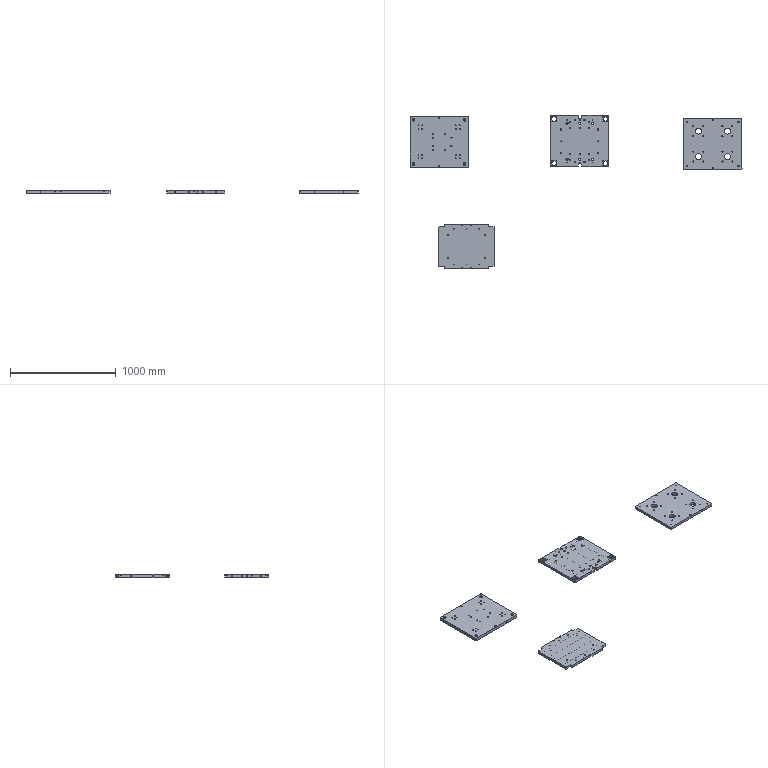NC program | Mastercam | posted with a generic post | part box 3140 x 1452 x 30 mm
Lines 17234 to 18407 of 22248, first 1084 of 1174 lines:
N4000 T12 M6
N4010 G0 G90 G17 G54 X-256.12 Y210.2 A0. S6000 M3
N4020 G43 H12 Z50. M8
N4030 Z1.
N4040 G1 Z-24.85 F600.
N4050 X-257.32 F1000.
N4060 G3 X-258.52 Y209. I0. J-1.2
N4070 X-242. Y192.48 I16.52 J0.
N4080 X-225.48 Y209. I0. J16.52
N4090 X-242. Y225.52 I-16.52 J0.
N4100 X-258.52 Y209. I0. J-16.52
N4110 X-258.512 Y208.5 I16.52 J0.
N4120 X-257.313 Y207.336 I1.199 J.036
N4130 X-257.277 Y207.337 I0. J1.2
N4140 G1 X-256.077 Y207.373
N4150 X-256.14 Y210.2
N4160 X-257.34
N4170 G3 X-258.54 Y209. I0. J-1.2
N4180 X-242. Y192.46 I16.54 J0.
N4190 X-225.46 Y209. I0. J16.54
N4200 X-242. Y225.54 I-16.54 J0.
N4210 X-258.54 Y209. I0. J-16.54
N4220 X-258.532 Y208.5 I16.54 J0.
N4230 X-257.333 Y207.336 I1.199 J.036
N4240 X-257.297 Y207.337 I0. J1.2
N4250 G1 X-256.097 Y207.373
N4260 G0 Z50.
N4270 X227.88 Y210.2
N4280 Z1.
N4290 G1 Z-24.85 F600.
N4300 X226.68 F1000.
N4310 G3 X225.48 Y209. I0. J-1.2
N4320 X242. Y192.48 I16.52 J0.
N4330 X258.52 Y209. I0. J16.52
N4340 X242. Y225.52 I-16.52 J0.
N4350 X225.48 Y209. I0. J-16.52
N4360 X225.488 Y208.5 I16.52 J0.
N4370 X226.687 Y207.336 I1.199 J.036
N4380 X226.723 Y207.337 I0. J1.2
N4390 G1 X227.923 Y207.373
N4400 X227.86 Y210.2
N4410 X226.66
N4420 G3 X225.46 Y209. I0. J-1.2
N4430 X242. Y192.46 I16.54 J0.
N4440 X258.54 Y209. I0. J16.54
N4450 X242. Y225.54 I-16.54 J0.
N4460 X225.46 Y209. I0. J-16.54
N4470 X225.468 Y208.5 I16.54 J0.
N4480 X226.667 Y207.336 I1.199 J.036
N4490 X226.703 Y207.337 I0. J1.2
N4500 G1 X227.903 Y207.373
N4510 G0 Z50.
N4520 X227.88 Y-207.8
N4530 Z1.
N4540 G1 Z-24.85 F600.
N4550 X226.68 F1000.
N4560 G3 X225.48 Y-209. I0. J-1.2
N4570 X242. Y-225.52 I16.52 J0.
N4580 X258.52 Y-209. I0. J16.52
N4590 X242. Y-192.48 I-16.52 J0.
N4600 X225.48 Y-209. I0. J-16.52
N4610 X225.488 Y-209.5 I16.52 J0.
N4620 X226.687 Y-210.664 I1.199 J.036
N4630 X226.723 Y-210.663 I0. J1.2
N4640 G1 X227.923 Y-210.627
N4650 X227.86 Y-207.8
N4660 X226.66
N4670 G3 X225.46 Y-209. I0. J-1.2
N4680 X242. Y-225.54 I16.54 J0.
N4690 X258.54 Y-209. I0. J16.54
N4700 X242. Y-192.46 I-16.54 J0.
N4710 X225.46 Y-209. I0. J-16.54
N4720 X225.468 Y-209.5 I16.54 J0.
N4730 X226.667 Y-210.664 I1.199 J.036
N4740 X226.703 Y-210.663 I0. J1.2
N4750 G1 X227.903 Y-210.627
N4760 G0 Z50.
N4770 X-256.12 Y-207.8
N4780 Z1.
N4790 G1 Z-24.85 F600.
N4800 X-257.32 F1000.
N4810 G3 X-258.52 Y-209. I0. J-1.2
N4820 X-242. Y-225.52 I16.52 J0.
N4830 X-225.48 Y-209. I0. J16.52
N4840 X-242. Y-192.48 I-16.52 J0.
N4850 X-258.52 Y-209. I0. J-16.52
N4860 X-258.512 Y-209.5 I16.52 J0.
N4870 X-257.313 Y-210.664 I1.199 J.036
N4880 X-257.277 Y-210.663 I0. J1.2
N4890 G1 X-256.077 Y-210.627
N4900 X-256.14 Y-207.8
N4910 X-257.34
N4920 G3 X-258.54 Y-209. I0. J-1.2
N4930 X-242. Y-225.54 I16.54 J0.
N4940 X-225.46 Y-209. I0. J16.54
N4950 X-242. Y-192.46 I-16.54 J0.
N4960 X-258.54 Y-209. I0. J-16.54
N4970 X-258.532 Y-209.5 I16.54 J0.
N4980 X-257.333 Y-210.664 I1.199 J.036
N4990 X-257.297 Y-210.663 I0. J1.2
N5000 G1 X-256.097 Y-210.627
N5010 G0 Z50.
N5020 X-124.18 Y170.
N5030 Z1.2
N5040 G1 Z.2 F600.
N5050 G3 X-120. Y165.82 Z.025 I4.18 J0. F2000.
N5060 X-115.82 Y170. Z-.15 I0. J4.18
N5070 X-120. Y174.18 Z-.325 I-4.18 J0.
N5080 X-124.18 Y170. Z-.5 I0. J-4.18
N5090 X-120. Y165.82 Z-.675 I4.18 J0.
N5100 X-115.82 Y170. Z-.85 I0. J4.18
N5110 X-120. Y174.18 Z-1.025 I-4.18 J0.
N5120 X-124.18 Y170. Z-1.2 I0. J-4.18
N5130 X-120. Y165.82 Z-1.375 I4.18 J0.
N5140 X-115.82 Y170. Z-1.55 I0. J4.18
N5150 X-120. Y174.18 Z-1.725 I-4.18 J0.
N5160 X-124.18 Y170. Z-1.9 I0. J-4.18
N5170 X-120. Y165.82 Z-2.075 I4.18 J0.
N5180 X-115.82 Y170. Z-2.25 I0. J4.18
N5190 X-120. Y174.18 Z-2.425 I-4.18 J0.
N5200 X-124.18 Y170. Z-2.6 I0. J-4.18
N5210 X-120. Y165.82 Z-2.775 I4.18 J0.
N5220 X-115.82 Y170. Z-2.95 I0. J4.18
N5230 X-120. Y174.18 Z-3.125 I-4.18 J0.
N5240 X-124.18 Y170. Z-3.3 I0. J-4.18
N5250 X-120. Y165.82 Z-3.475 I4.18 J0.
N5260 X-115.82 Y170. Z-3.65 I0. J4.18
N5270 X-120. Y174.18 Z-3.825 I-4.18 J0.
N5280 X-124.18 Y170. Z-4. I0. J-4.18
N5290 X-120. Y165.82 Z-4.175 I4.18 J0.
N5300 X-115.82 Y170. Z-4.35 I0. J4.18
N5310 X-120. Y174.18 Z-4.525 I-4.18 J0.
N5320 X-124.18 Y170. Z-4.7 I0. J-4.18
N5330 X-120. Y165.82 Z-4.875 I4.18 J0.
N5340 X-115.82 Y170. Z-5.05 I0. J4.18
N5350 X-120. Y174.18 Z-5.225 I-4.18 J0.
N5360 X-124.18 Y170. Z-5.4 I0. J-4.18
N5370 X-120. Y165.82 Z-5.575 I4.18 J0.
N5380 X-115.82 Y170. Z-5.75 I0. J4.18
N5390 X-120. Y174.18 Z-5.925 I-4.18 J0.
N5400 X-124.18 Y170. Z-6.1 I0. J-4.18
N5410 X-120. Y165.82 Z-6.275 I4.18 J0.
N5420 X-115.82 Y170. Z-6.45 I0. J4.18
N5430 X-120. Y174.18 Z-6.625 I-4.18 J0.
N5440 X-124.18 Y170. Z-6.8 I0. J-4.18
N5450 X-120. Y165.82 Z-6.975 I4.18 J0.
N5460 X-115.82 Y170. Z-7.15 I0. J4.18
N5470 X-120. Y174.18 Z-7.325 I-4.18 J0.
N5480 X-124.18 Y170. Z-7.5 I0. J-4.18
N5490 X-120. Y165.82 Z-7.675 I4.18 J0.
N5500 X-115.82 Y170. Z-7.85 I0. J4.18
N5510 X-120. Y174.18 Z-8.025 I-4.18 J0.
N5520 X-124.18 Y170. Z-8.2 I0. J-4.18
N5530 X-120. Y165.82 Z-8.375 I4.18 J0.
N5540 X-115.82 Y170. Z-8.55 I0. J4.18
N5550 X-120. Y174.18 Z-8.725 I-4.18 J0.
N5560 X-124.18 Y170. Z-8.9 I0. J-4.18
N5570 X-120. Y165.82 Z-9.075 I4.18 J0.
N5580 X-115.82 Y170. Z-9.25 I0. J4.18
N5590 X-120. Y174.18 Z-9.425 I-4.18 J0.
N5600 X-124.18 Y170. Z-9.6 I0. J-4.18
N5610 X-120. Y165.82 Z-9.775 I4.18 J0.
N5620 X-115.82 Y170. Z-9.95 I0. J4.18
N5630 X-120. Y174.18 Z-10.125 I-4.18 J0.
N5640 X-124.18 Y170. Z-10.3 I0. J-4.18
N5650 X-120. Y165.82 Z-10.475 I4.18 J0.
N5660 X-115.82 Y170. Z-10.65 I0. J4.18
N5670 X-120. Y174.18 Z-10.825 I-4.18 J0.
N5680 X-124.18 Y170. Z-11. I0. J-4.18
N5690 X-120. Y165.82 Z-11.175 I4.18 J0.
N5700 X-115.82 Y170. Z-11.35 I0. J4.18
N5710 X-120. Y174.18 Z-11.525 I-4.18 J0.
N5720 X-124.18 Y170. Z-11.7 I0. J-4.18
N5730 X-120. Y165.82 Z-11.875 I4.18 J0.
N5740 X-115.82 Y170. Z-12.05 I0. J4.18
N5750 X-120. Y174.18 Z-12.225 I-4.18 J0.
N5760 X-124.18 Y170. Z-12.4 I0. J-4.18
N5770 X-120. Y165.82 Z-12.575 I4.18 J0.
N5780 X-115.82 Y170. Z-12.75 I0. J4.18
N5790 X-120. Y174.18 Z-12.925 I-4.18 J0.
N5800 X-124.18 Y170. Z-13.1 I0. J-4.18
N5810 X-120. Y165.82 Z-13.275 I4.18 J0.
N5820 X-115.82 Y170. Z-13.45 I0. J4.18
N5830 X-120. Y174.18 Z-13.625 I-4.18 J0.
N5840 X-124.18 Y170. Z-13.8 I0. J-4.18
N5850 X-120. Y165.82 Z-13.975 I4.18 J0.
N5860 X-115.82 Y170. Z-14.15 I0. J4.18
N5870 X-120. Y174.18 Z-14.325 I-4.18 J0.
N5880 X-124.18 Y170. Z-14.5 I0. J-4.18
N5890 X-120. Y165.82 Z-14.675 I4.18 J0.
N5900 X-115.82 Y170. Z-14.85 I0. J4.18
N5910 X-120. Y174.18 Z-15.025 I-4.18 J0.
N5920 X-124.18 Y170. Z-15.2 I0. J-4.18
N5930 X-120. Y165.82 Z-15.375 I4.18 J0.
N5940 X-115.82 Y170. Z-15.55 I0. J4.18
N5950 X-120. Y174.18 Z-15.725 I-4.18 J0.
N5960 X-124.18 Y170. Z-15.9 I0. J-4.18
N5970 X-120. Y165.82 Z-16.075 I4.18 J0.
N5980 X-115.82 Y170. Z-16.25 I0. J4.18
N5990 X-120. Y174.18 Z-16.425 I-4.18 J0.
N6000 X-124.18 Y170. Z-16.6 I0. J-4.18
N6010 X-120. Y165.82 Z-16.775 I4.18 J0.
N6020 X-115.82 Y170. Z-16.95 I0. J4.18
N6030 X-120. Y174.18 Z-17.125 I-4.18 J0.
N6040 X-124.18 Y170. Z-17.3 I0. J-4.18
N6050 X-120. Y165.82 Z-17.475 I4.18 J0.
N6060 X-115.82 Y170. Z-17.65 I0. J4.18
N6070 X-120. Y174.18 Z-17.825 I-4.18 J0.
N6080 X-124.18 Y170. Z-18. I0. J-4.18
N6090 X-120. Y165.82 Z-18.175 I4.18 J0.
N6100 X-115.82 Y170. Z-18.35 I0. J4.18
N6110 X-120. Y174.18 Z-18.525 I-4.18 J0.
N6120 X-124.18 Y170. Z-18.7 I0. J-4.18
N6130 X-120. Y165.82 Z-18.875 I4.18 J0.
N6140 X-115.82 Y170. Z-19.05 I0. J4.18
N6150 X-120. Y174.18 Z-19.225 I-4.18 J0.
N6160 X-124.18 Y170. Z-19.4 I0. J-4.18
N6170 X-120. Y165.82 Z-19.575 I4.18 J0.
N6180 X-115.82 Y170. Z-19.75 I0. J4.18
N6190 X-120. Y174.18 Z-19.925 I-4.18 J0.
N6200 X-124.18 Y170. Z-20.1 I0. J-4.18
N6210 X-120. Y165.82 Z-20.275 I4.18 J0.
N6220 X-115.82 Y170. Z-20.45 I0. J4.18
N6230 X-120. Y174.18 Z-20.625 I-4.18 J0.
N6240 X-124.18 Y170. Z-20.8 I0. J-4.18
N6250 X-120. Y165.82 Z-20.975 I4.18 J0.
N6260 X-115.82 Y170. Z-21.15 I0. J4.18
N6270 X-120. Y174.18 Z-21.325 I-4.18 J0.
N6280 X-124.18 Y170. Z-21.5 I0. J-4.18
N6290 X-120. Y165.82 Z-21.675 I4.18 J0.
N6300 X-115.82 Y170. Z-21.85 I0. J4.18
N6310 X-120. Y174.18 Z-22.025 I-4.18 J0.
N6320 X-124.18 Y170. Z-22.2 I0. J-4.18
N6330 X-120. Y165.82 Z-22.375 I4.18 J0.
N6340 X-115.82 Y170. Z-22.55 I0. J4.18
N6350 X-120. Y174.18 Z-22.725 I-4.18 J0.
N6360 X-124.18 Y170. Z-22.9 I0. J-4.18
N6370 X-120. Y165.82 Z-23.075 I4.18 J0.
N6380 X-115.82 Y170. Z-23.25 I0. J4.18
N6390 X-120. Y174.18 Z-23.425 I-4.18 J0.
N6400 X-124.18 Y170. Z-23.6 I0. J-4.18
N6410 X-120. Y165.82 Z-23.775 I4.18 J0.
N6420 X-115.82 Y170. Z-23.95 I0. J4.18
N6430 X-120. Y174.18 Z-24.125 I-4.18 J0.
N6440 X-124.18 Y170. Z-24.3 I0. J-4.18
N6450 X-120. Y165.82 Z-24.475 I4.18 J0.
N6460 X-115.82 Y170. Z-24.65 I0. J4.18
N6470 X-120. Y174.18 Z-24.825 I-4.18 J0.
N6480 X-120.93 Y174.075 Z-24.85 I0. J-4.18
N6490 X-124.18 Y170. I.93 J-4.075
N6500 X-120. Y165.82 I4.18 J0.
N6510 X-115.82 Y170. I0. J4.18
N6520 X-120. Y174.18 I-4.18 J0.
N6530 X-121.41 Y173.935 I0. J-4.18
N6540 G0 Z50.
N6550 X-4.18 Y170.
N6560 Z1.2
N6570 G1 Z.2 F600.
N6580 G3 X0. Y165.82 Z.025 I4.18 J0. F2000.
N6590 X4.18 Y170. Z-.15 I0. J4.18
N6600 X0. Y174.18 Z-.325 I-4.18 J0.
N6610 X-4.18 Y170. Z-.5 I0. J-4.18
N6620 X0. Y165.82 Z-.675 I4.18 J0.
N6630 X4.18 Y170. Z-.85 I0. J4.18
N6640 X0. Y174.18 Z-1.025 I-4.18 J0.
N6650 X-4.18 Y170. Z-1.2 I0. J-4.18
N6660 X0. Y165.82 Z-1.375 I4.18 J0.
N6670 X4.18 Y170. Z-1.55 I0. J4.18
N6680 X0. Y174.18 Z-1.725 I-4.18 J0.
N6690 X-4.18 Y170. Z-1.9 I0. J-4.18
N6700 X0. Y165.82 Z-2.075 I4.18 J0.
N6710 X4.18 Y170. Z-2.25 I0. J4.18
N6720 X0. Y174.18 Z-2.425 I-4.18 J0.
N6730 X-4.18 Y170. Z-2.6 I0. J-4.18
N6740 X0. Y165.82 Z-2.775 I4.18 J0.
N6750 X4.18 Y170. Z-2.95 I0. J4.18
N6760 X0. Y174.18 Z-3.125 I-4.18 J0.
N6770 X-4.18 Y170. Z-3.3 I0. J-4.18
N6780 X0. Y165.82 Z-3.475 I4.18 J0.
N6790 X4.18 Y170. Z-3.65 I0. J4.18
N6800 X0. Y174.18 Z-3.825 I-4.18 J0.
N6810 X-4.18 Y170. Z-4. I0. J-4.18
N6820 X0. Y165.82 Z-4.175 I4.18 J0.
N6830 X4.18 Y170. Z-4.35 I0. J4.18
N6840 X0. Y174.18 Z-4.525 I-4.18 J0.
N6850 X-4.18 Y170. Z-4.7 I0. J-4.18
N6860 X0. Y165.82 Z-4.875 I4.18 J0.
N6870 X4.18 Y170. Z-5.05 I0. J4.18
N6880 X0. Y174.18 Z-5.225 I-4.18 J0.
N6890 X-4.18 Y170. Z-5.4 I0. J-4.18
N6900 X0. Y165.82 Z-5.575 I4.18 J0.
N6910 X4.18 Y170. Z-5.75 I0. J4.18
N6920 X0. Y174.18 Z-5.925 I-4.18 J0.
N6930 X-4.18 Y170. Z-6.1 I0. J-4.18
N6940 X0. Y165.82 Z-6.275 I4.18 J0.
N6950 X4.18 Y170. Z-6.45 I0. J4.18
N6960 X0. Y174.18 Z-6.625 I-4.18 J0.
N6970 X-4.18 Y170. Z-6.8 I0. J-4.18
N6980 X0. Y165.82 Z-6.975 I4.18 J0.
N6990 X4.18 Y170. Z-7.15 I0. J4.18
N7000 X0. Y174.18 Z-7.325 I-4.18 J0.
N7010 X-4.18 Y170. Z-7.5 I0. J-4.18
N7020 X0. Y165.82 Z-7.675 I4.18 J0.
N7030 X4.18 Y170. Z-7.85 I0. J4.18
N7040 X0. Y174.18 Z-8.025 I-4.18 J0.
N7050 X-4.18 Y170. Z-8.2 I0. J-4.18
N7060 X0. Y165.82 Z-8.375 I4.18 J0.
N7070 X4.18 Y170. Z-8.55 I0. J4.18
N7080 X0. Y174.18 Z-8.725 I-4.18 J0.
N7090 X-4.18 Y170. Z-8.9 I0. J-4.18
N7100 X0. Y165.82 Z-9.075 I4.18 J0.
N7110 X4.18 Y170. Z-9.25 I0. J4.18
N7120 X0. Y174.18 Z-9.425 I-4.18 J0.
N7130 X-4.18 Y170. Z-9.6 I0. J-4.18
N7140 X0. Y165.82 Z-9.775 I4.18 J0.
N7150 X4.18 Y170. Z-9.95 I0. J4.18
N7160 X0. Y174.18 Z-10.125 I-4.18 J0.
N7170 X-4.18 Y170. Z-10.3 I0. J-4.18
N7180 X0. Y165.82 Z-10.475 I4.18 J0.
N7190 X4.18 Y170. Z-10.65 I0. J4.18
N7200 X0. Y174.18 Z-10.825 I-4.18 J0.
N7210 X-4.18 Y170. Z-11. I0. J-4.18
N7220 X0. Y165.82 Z-11.175 I4.18 J0.
N7230 X4.18 Y170. Z-11.35 I0. J4.18
N7240 X0. Y174.18 Z-11.525 I-4.18 J0.
N7250 X-4.18 Y170. Z-11.7 I0. J-4.18
N7260 X0. Y165.82 Z-11.875 I4.18 J0.
N7270 X4.18 Y170. Z-12.05 I0. J4.18
N7280 X0. Y174.18 Z-12.225 I-4.18 J0.
N7290 X-4.18 Y170. Z-12.4 I0. J-4.18
N7300 X0. Y165.82 Z-12.575 I4.18 J0.
N7310 X4.18 Y170. Z-12.75 I0. J4.18
N7320 X0. Y174.18 Z-12.925 I-4.18 J0.
N7330 X-4.18 Y170. Z-13.1 I0. J-4.18
N7340 X0. Y165.82 Z-13.275 I4.18 J0.
N7350 X4.18 Y170. Z-13.45 I0. J4.18
N7360 X0. Y174.18 Z-13.625 I-4.18 J0.
N7370 X-4.18 Y170. Z-13.8 I0. J-4.18
N7380 X0. Y165.82 Z-13.975 I4.18 J0.
N7390 X4.18 Y170. Z-14.15 I0. J4.18
N7400 X0. Y174.18 Z-14.325 I-4.18 J0.
N7410 X-4.18 Y170. Z-14.5 I0. J-4.18
N7420 X0. Y165.82 Z-14.675 I4.18 J0.
N7430 X4.18 Y170. Z-14.85 I0. J4.18
N7440 X0. Y174.18 Z-15.025 I-4.18 J0.
N7450 X-4.18 Y170. Z-15.2 I0. J-4.18
N7460 X0. Y165.82 Z-15.375 I4.18 J0.
N7470 X4.18 Y170. Z-15.55 I0. J4.18
N7480 X0. Y174.18 Z-15.725 I-4.18 J0.
N7490 X-4.18 Y170. Z-15.9 I0. J-4.18
N7500 X0. Y165.82 Z-16.075 I4.18 J0.
N7510 X4.18 Y170. Z-16.25 I0. J4.18
N7520 X0. Y174.18 Z-16.425 I-4.18 J0.
N7530 X-4.18 Y170. Z-16.6 I0. J-4.18
N7540 X0. Y165.82 Z-16.775 I4.18 J0.
N7550 X4.18 Y170. Z-16.95 I0. J4.18
N7560 X0. Y174.18 Z-17.125 I-4.18 J0.
N7570 X-4.18 Y170. Z-17.3 I0. J-4.18
N7580 X0. Y165.82 Z-17.475 I4.18 J0.
N7590 X4.18 Y170. Z-17.65 I0. J4.18
N7600 X0. Y174.18 Z-17.825 I-4.18 J0.
N7610 X-4.18 Y170. Z-18. I0. J-4.18
N7620 X0. Y165.82 Z-18.175 I4.18 J0.
N7630 X4.18 Y170. Z-18.35 I0. J4.18
N7640 X0. Y174.18 Z-18.525 I-4.18 J0.
N7650 X-4.18 Y170. Z-18.7 I0. J-4.18
N7660 X0. Y165.82 Z-18.875 I4.18 J0.
N7670 X4.18 Y170. Z-19.05 I0. J4.18
N7680 X0. Y174.18 Z-19.225 I-4.18 J0.
N7690 X-4.18 Y170. Z-19.4 I0. J-4.18
N7700 X0. Y165.82 Z-19.575 I4.18 J0.
N7710 X4.18 Y170. Z-19.75 I0. J4.18
N7720 X0. Y174.18 Z-19.925 I-4.18 J0.
N7730 X-4.18 Y170. Z-20.1 I0. J-4.18
N7740 X0. Y165.82 Z-20.275 I4.18 J0.
N7750 X4.18 Y170. Z-20.45 I0. J4.18
N7760 X0. Y174.18 Z-20.625 I-4.18 J0.
N7770 X-4.18 Y170. Z-20.8 I0. J-4.18
N7780 X0. Y165.82 Z-20.975 I4.18 J0.
N7790 X4.18 Y170. Z-21.15 I0. J4.18
N7800 X0. Y174.18 Z-21.325 I-4.18 J0.
N7810 X-4.18 Y170. Z-21.5 I0. J-4.18
N7820 X0. Y165.82 Z-21.675 I4.18 J0.
N7830 X4.18 Y170. Z-21.85 I0. J4.18
N7840 X0. Y174.18 Z-22.025 I-4.18 J0.
N7850 X-4.18 Y170. Z-22.2 I0. J-4.18
N7860 X0. Y165.82 Z-22.375 I4.18 J0.
N7870 X4.18 Y170. Z-22.55 I0. J4.18
N7880 X0. Y174.18 Z-22.725 I-4.18 J0.
N7890 X-4.18 Y170. Z-22.9 I0. J-4.18
N7900 X0. Y165.82 Z-23.075 I4.18 J0.
N7910 X4.18 Y170. Z-23.25 I0. J4.18
N7920 X0. Y174.18 Z-23.425 I-4.18 J0.
N7930 X-4.18 Y170. Z-23.6 I0. J-4.18
N7940 X0. Y165.82 Z-23.775 I4.18 J0.
N7950 X4.18 Y170. Z-23.95 I0. J4.18
N7960 X0. Y174.18 Z-24.125 I-4.18 J0.
N7970 X-4.18 Y170. Z-24.3 I0. J-4.18
N7980 X0. Y165.82 Z-24.475 I4.18 J0.
N7990 X4.18 Y170. Z-24.65 I0. J4.18
N8000 X0. Y174.18 Z-24.825 I-4.18 J0.
N8010 X-.93 Y174.075 Z-24.85 I0. J-4.18
N8020 X-4.18 Y170. I.93 J-4.075
N8030 X0. Y165.82 I4.18 J0.
N8040 X4.18 Y170. I0. J4.18
N8050 X0. Y174.18 I-4.18 J0.
N8060 X-1.41 Y173.935 I0. J-4.18
N8070 G0 Z50.
N8080 X115.82 Y170.
N8090 Z1.2
N8100 G1 Z.2 F600.
N8110 G3 X120. Y165.82 Z.025 I4.18 J0. F2000.
N8120 X124.18 Y170. Z-.15 I0. J4.18
N8130 X120. Y174.18 Z-.325 I-4.18 J0.
N8140 X115.82 Y170. Z-.5 I0. J-4.18
N8150 X120. Y165.82 Z-.675 I4.18 J0.
N8160 X124.18 Y170. Z-.85 I0. J4.18
N8170 X120. Y174.18 Z-1.025 I-4.18 J0.
N8180 X115.82 Y170. Z-1.2 I0. J-4.18
N8190 X120. Y165.82 Z-1.375 I4.18 J0.
N8200 X124.18 Y170. Z-1.55 I0. J4.18
N8210 X120. Y174.18 Z-1.725 I-4.18 J0.
N8220 X115.82 Y170. Z-1.9 I0. J-4.18
N8230 X120. Y165.82 Z-2.075 I4.18 J0.
N8240 X124.18 Y170. Z-2.25 I0. J4.18
N8250 X120. Y174.18 Z-2.425 I-4.18 J0.
N8260 X115.82 Y170. Z-2.6 I0. J-4.18
N8270 X120. Y165.82 Z-2.775 I4.18 J0.
N8280 X124.18 Y170. Z-2.95 I0. J4.18
N8290 X120. Y174.18 Z-3.125 I-4.18 J0.
N8300 X115.82 Y170. Z-3.3 I0. J-4.18
N8310 X120. Y165.82 Z-3.475 I4.18 J0.
N8320 X124.18 Y170. Z-3.65 I0. J4.18
N8330 X120. Y174.18 Z-3.825 I-4.18 J0.
N8340 X115.82 Y170. Z-4. I0. J-4.18
N8350 X120. Y165.82 Z-4.175 I4.18 J0.
N8360 X124.18 Y170. Z-4.35 I0. J4.18
N8370 X120. Y174.18 Z-4.525 I-4.18 J0.
N8380 X115.82 Y170. Z-4.7 I0. J-4.18
N8390 X120. Y165.82 Z-4.875 I4.18 J0.
N8400 X124.18 Y170. Z-5.05 I0. J4.18
N8410 X120. Y174.18 Z-5.225 I-4.18 J0.
N8420 X115.82 Y170. Z-5.4 I0. J-4.18
N8430 X120. Y165.82 Z-5.575 I4.18 J0.
N8440 X124.18 Y170. Z-5.75 I0. J4.18
N8450 X120. Y174.18 Z-5.925 I-4.18 J0.
N8460 X115.82 Y170. Z-6.1 I0. J-4.18
N8470 X120. Y165.82 Z-6.275 I4.18 J0.
N8480 X124.18 Y170. Z-6.45 I0. J4.18
N8490 X120. Y174.18 Z-6.625 I-4.18 J0.
N8500 X115.82 Y170. Z-6.8 I0. J-4.18
N8510 X120. Y165.82 Z-6.975 I4.18 J0.
N8520 X124.18 Y170. Z-7.15 I0. J4.18
N8530 X120. Y174.18 Z-7.325 I-4.18 J0.
N8540 X115.82 Y170. Z-7.5 I0. J-4.18
N8550 X120. Y165.82 Z-7.675 I4.18 J0.
N8560 X124.18 Y170. Z-7.85 I0. J4.18
N8570 X120. Y174.18 Z-8.025 I-4.18 J0.
N8580 X115.82 Y170. Z-8.2 I0. J-4.18
N8590 X120. Y165.82 Z-8.375 I4.18 J0.
N8600 X124.18 Y170. Z-8.55 I0. J4.18
N8610 X120. Y174.18 Z-8.725 I-4.18 J0.
N8620 X115.82 Y170. Z-8.9 I0. J-4.18
N8630 X120. Y165.82 Z-9.075 I4.18 J0.
N8640 X124.18 Y170. Z-9.25 I0. J4.18
N8650 X120. Y174.18 Z-9.425 I-4.18 J0.
N8660 X115.82 Y170. Z-9.6 I0. J-4.18
N8670 X120. Y165.82 Z-9.775 I4.18 J0.
N8680 X124.18 Y170. Z-9.95 I0. J4.18
N8690 X120. Y174.18 Z-10.125 I-4.18 J0.
N8700 X115.82 Y170. Z-10.3 I0. J-4.18
N8710 X120. Y165.82 Z-10.475 I4.18 J0.
N8720 X124.18 Y170. Z-10.65 I0. J4.18
N8730 X120. Y174.18 Z-10.825 I-4.18 J0.
N8740 X115.82 Y170. Z-11. I0. J-4.18
N8750 X120. Y165.82 Z-11.175 I4.18 J0.
N8760 X124.18 Y170. Z-11.35 I0. J4.18
N8770 X120. Y174.18 Z-11.525 I-4.18 J0.
N8780 X115.82 Y170. Z-11.7 I0. J-4.18
N8790 X120. Y165.82 Z-11.875 I4.18 J0.
N8800 X124.18 Y170. Z-12.05 I0. J4.18
N8810 X120. Y174.18 Z-12.225 I-4.18 J0.
N8820 X115.82 Y170. Z-12.4 I0. J-4.18
N8830 X120. Y165.82 Z-12.575 I4.18 J0.
N8840 X124.18 Y170. Z-12.75 I0. J4.18
N8850 X120. Y174.18 Z-12.925 I-4.18 J0.
N8860 X115.82 Y170. Z-13.1 I0. J-4.18
N8870 X120. Y165.82 Z-13.275 I4.18 J0.
N8880 X124.18 Y170. Z-13.45 I0. J4.18
N8890 X120. Y174.18 Z-13.625 I-4.18 J0.
N8900 X115.82 Y170. Z-13.8 I0. J-4.18
N8910 X120. Y165.82 Z-13.975 I4.18 J0.
N8920 X124.18 Y170. Z-14.15 I0. J4.18
N8930 X120. Y174.18 Z-14.325 I-4.18 J0.
N8940 X115.82 Y170. Z-14.5 I0. J-4.18
N8950 X120. Y165.82 Z-14.675 I4.18 J0.
N8960 X124.18 Y170. Z-14.85 I0. J4.18
N8970 X120. Y174.18 Z-15.025 I-4.18 J0.
N8980 X115.82 Y170. Z-15.2 I0. J-4.18
N8990 X120. Y165.82 Z-15.375 I4.18 J0.
N9000 X124.18 Y170. Z-15.55 I0. J4.18
N9010 X120. Y174.18 Z-15.725 I-4.18 J0.
N9020 X115.82 Y170. Z-15.9 I0. J-4.18
N9030 X120. Y165.82 Z-16.075 I4.18 J0.
N9040 X124.18 Y170. Z-16.25 I0. J4.18
N9050 X120. Y174.18 Z-16.425 I-4.18 J0.
N9060 X115.82 Y170. Z-16.6 I0. J-4.18
N9070 X120. Y165.82 Z-16.775 I4.18 J0.
N9080 X124.18 Y170. Z-16.95 I0. J4.18
N9090 X120. Y174.18 Z-17.125 I-4.18 J0.
N9100 X115.82 Y170. Z-17.3 I0. J-4.18
N9110 X120. Y165.82 Z-17.475 I4.18 J0.
N9120 X124.18 Y170. Z-17.65 I0. J4.18
N9130 X120. Y174.18 Z-17.825 I-4.18 J0.
N9140 X115.82 Y170. Z-18. I0. J-4.18
N9150 X120. Y165.82 Z-18.175 I4.18 J0.
N9160 X124.18 Y170. Z-18.35 I0. J4.18
N9170 X120. Y174.18 Z-18.525 I-4.18 J0.
N9180 X115.82 Y170. Z-18.7 I0. J-4.18
N9190 X120. Y165.82 Z-18.875 I4.18 J0.
N9200 X124.18 Y170. Z-19.05 I0. J4.18
N9210 X120. Y174.18 Z-19.225 I-4.18 J0.
N9220 X115.82 Y170. Z-19.4 I0. J-4.18
N9230 X120. Y165.82 Z-19.575 I4.18 J0.
N9240 X124.18 Y170. Z-19.75 I0. J4.18
N9250 X120. Y174.18 Z-19.925 I-4.18 J0.
N9260 X115.82 Y170. Z-20.1 I0. J-4.18
N9270 X120. Y165.82 Z-20.275 I4.18 J0.
N9280 X124.18 Y170. Z-20.45 I0. J4.18
N9290 X120. Y174.18 Z-20.625 I-4.18 J0.
N9300 X115.82 Y170. Z-20.8 I0. J-4.18
N9310 X120. Y165.82 Z-20.975 I4.18 J0.
N9320 X124.18 Y170. Z-21.15 I0. J4.18
N9330 X120. Y174.18 Z-21.325 I-4.18 J0.
N9340 X115.82 Y170. Z-21.5 I0. J-4.18
N9350 X120. Y165.82 Z-21.675 I4.18 J0.
N9360 X124.18 Y170. Z-21.85 I0. J4.18
N9370 X120. Y174.18 Z-22.025 I-4.18 J0.
N9380 X115.82 Y170. Z-22.2 I0. J-4.18
N9390 X120. Y165.82 Z-22.375 I4.18 J0.
N9400 X124.18 Y170. Z-22.55 I0. J4.18
N9410 X120. Y174.18 Z-22.725 I-4.18 J0.
N9420 X115.82 Y170. Z-22.9 I0. J-4.18
N9430 X120. Y165.82 Z-23.075 I4.18 J0.
N9440 X124.18 Y170. Z-23.25 I0. J4.18
N9450 X120. Y174.18 Z-23.425 I-4.18 J0.
N9460 X115.82 Y170. Z-23.6 I0. J-4.18
N9470 X120. Y165.82 Z-23.775 I4.18 J0.
N9480 X124.18 Y170. Z-23.95 I0. J4.18
N9490 X120. Y174.18 Z-24.125 I-4.18 J0.
N9500 X115.82 Y170. Z-24.3 I0. J-4.18
N9510 X120. Y165.82 Z-24.475 I4.18 J0.
N9520 X124.18 Y170. Z-24.65 I0. J4.18
N9530 X120. Y174.18 Z-24.825 I-4.18 J0.
N9540 X119.07 Y174.075 Z-24.85 I0. J-4.18
N9550 X115.82 Y170. I.93 J-4.075
N9560 X120. Y165.82 I4.18 J0.
N9570 X124.18 Y170. I0. J4.18
N9580 X120. Y174.18 I-4.18 J0.
N9590 X118.59 Y173.935 I0. J-4.18
N9600 G0 Z50.
N9610 X115.82 Y-170.
N9620 Z1.2
N9630 G1 Z.2 F600.
N9640 G3 X120. Y-174.18 Z.025 I4.18 J0. F2000.
N9650 X124.18 Y-170. Z-.15 I0. J4.18
N9660 X120. Y-165.82 Z-.325 I-4.18 J0.
N9670 X115.82 Y-170. Z-.5 I0. J-4.18
N9680 X120. Y-174.18 Z-.675 I4.18 J0.
N9690 X124.18 Y-170. Z-.85 I0. J4.18
N9700 X120. Y-165.82 Z-1.025 I-4.18 J0.
N9710 X115.82 Y-170. Z-1.2 I0. J-4.18
N9720 X120. Y-174.18 Z-1.375 I4.18 J0.
N9730 X124.18 Y-170. Z-1.55 I0. J4.18
N9740 X120. Y-165.82 Z-1.725 I-4.18 J0.
N9750 X115.82 Y-170. Z-1.9 I0. J-4.18
N9760 X120. Y-174.18 Z-2.075 I4.18 J0.
N9770 X124.18 Y-170. Z-2.25 I0. J4.18
N9780 X120. Y-165.82 Z-2.425 I-4.18 J0.
N9790 X115.82 Y-170. Z-2.6 I0. J-4.18
N9800 X120. Y-174.18 Z-2.775 I4.18 J0.
N9810 X124.18 Y-170. Z-2.95 I0. J4.18
N9820 X120. Y-165.82 Z-3.125 I-4.18 J0.
N9830 X115.82 Y-170. Z-3.3 I0. J-4.18
N9840 X120. Y-174.18 Z-3.475 I4.18 J0.
N9850 X124.18 Y-170. Z-3.65 I0. J4.18
N9860 X120. Y-165.82 Z-3.825 I-4.18 J0.
N9870 X115.82 Y-170. Z-4. I0. J-4.18
N9880 X120. Y-174.18 Z-4.175 I4.18 J0.
N9890 X124.18 Y-170. Z-4.35 I0. J4.18
N9900 X120. Y-165.82 Z-4.525 I-4.18 J0.
N9910 X115.82 Y-170. Z-4.7 I0. J-4.18
N9920 X120. Y-174.18 Z-4.875 I4.18 J0.
N9930 X124.18 Y-170. Z-5.05 I0. J4.18
N9940 X120. Y-165.82 Z-5.225 I-4.18 J0.
N9950 X115.82 Y-170. Z-5.4 I0. J-4.18
N9960 X120. Y-174.18 Z-5.575 I4.18 J0.
N9970 X124.18 Y-170. Z-5.75 I0. J4.18
N9980 X120. Y-165.82 Z-5.925 I-4.18 J0.
N9990 X115.82 Y-170. Z-6.1 I0. J-4.18
N100 X120. Y-174.18 Z-6.275 I4.18 J0.
N110 X124.18 Y-170. Z-6.45 I0. J4.18
N120 X120. Y-165.82 Z-6.625 I-4.18 J0.
N130 X115.82 Y-170. Z-6.8 I0. J-4.18
N140 X120. Y-174.18 Z-6.975 I4.18 J0.
N150 X124.18 Y-170. Z-7.15 I0. J4.18
N160 X120. Y-165.82 Z-7.325 I-4.18 J0.
N170 X115.82 Y-170. Z-7.5 I0. J-4.18
N180 X120. Y-174.18 Z-7.675 I4.18 J0.
N190 X124.18 Y-170. Z-7.85 I0. J4.18
N200 X120. Y-165.82 Z-8.025 I-4.18 J0.
N210 X115.82 Y-170. Z-8.2 I0. J-4.18
N220 X120. Y-174.18 Z-8.375 I4.18 J0.
N230 X124.18 Y-170. Z-8.55 I0. J4.18
N240 X120. Y-165.82 Z-8.725 I-4.18 J0.
N250 X115.82 Y-170. Z-8.9 I0. J-4.18
N260 X120. Y-174.18 Z-9.075 I4.18 J0.
N270 X124.18 Y-170. Z-9.25 I0. J4.18
N280 X120. Y-165.82 Z-9.425 I-4.18 J0.
N290 X115.82 Y-170. Z-9.6 I0. J-4.18
N300 X120. Y-174.18 Z-9.775 I4.18 J0.
N310 X124.18 Y-170. Z-9.95 I0. J4.18
N320 X120. Y-165.82 Z-10.125 I-4.18 J0.
N330 X115.82 Y-170. Z-10.3 I0. J-4.18
N340 X120. Y-174.18 Z-10.475 I4.18 J0.
N350 X124.18 Y-170. Z-10.65 I0. J4.18
N360 X120. Y-165.82 Z-10.825 I-4.18 J0.
N370 X115.82 Y-170. Z-11. I0. J-4.18
N380 X120. Y-174.18 Z-11.175 I4.18 J0.
N390 X124.18 Y-170. Z-11.35 I0. J4.18
N400 X120. Y-165.82 Z-11.525 I-4.18 J0.
N410 X115.82 Y-170. Z-11.7 I0. J-4.18
N420 X120. Y-174.18 Z-11.875 I4.18 J0.
N430 X124.18 Y-170. Z-12.05 I0. J4.18
N440 X120. Y-165.82 Z-12.225 I-4.18 J0.
N450 X115.82 Y-170. Z-12.4 I0. J-4.18
N460 X120. Y-174.18 Z-12.575 I4.18 J0.
N470 X124.18 Y-170. Z-12.75 I0. J4.18
N480 X120. Y-165.82 Z-12.925 I-4.18 J0.
N490 X115.82 Y-170. Z-13.1 I0. J-4.18
N500 X120. Y-174.18 Z-13.275 I4.18 J0.
N510 X124.18 Y-170. Z-13.45 I0. J4.18
N520 X120. Y-165.82 Z-13.625 I-4.18 J0.
N530 X115.82 Y-170. Z-13.8 I0. J-4.18
N540 X120. Y-174.18 Z-13.975 I4.18 J0.
N550 X124.18 Y-170. Z-14.15 I0. J4.18
N560 X120. Y-165.82 Z-14.325 I-4.18 J0.
N570 X115.82 Y-170. Z-14.5 I0. J-4.18
N580 X120. Y-174.18 Z-14.675 I4.18 J0.
N590 X124.18 Y-170. Z-14.85 I0. J4.18
N600 X120. Y-165.82 Z-15.025 I-4.18 J0.
N610 X115.82 Y-170. Z-15.2 I0. J-4.18
N620 X120. Y-174.18 Z-15.375 I4.18 J0.
N630 X124.18 Y-170. Z-15.55 I0. J4.18
N640 X120. Y-165.82 Z-15.725 I-4.18 J0.
N650 X115.82 Y-170. Z-15.9 I0. J-4.18
N660 X120. Y-174.18 Z-16.075 I4.18 J0.
N670 X124.18 Y-170. Z-16.25 I0. J4.18
N680 X120. Y-165.82 Z-16.425 I-4.18 J0.
N690 X115.82 Y-170. Z-16.6 I0. J-4.18
N700 X120. Y-174.18 Z-16.775 I4.18 J0.
N710 X124.18 Y-170. Z-16.95 I0. J4.18
N720 X120. Y-165.82 Z-17.125 I-4.18 J0.
N730 X115.82 Y-170. Z-17.3 I0. J-4.18
N740 X120. Y-174.18 Z-17.475 I4.18 J0.
N750 X124.18 Y-170. Z-17.65 I0. J4.18
N760 X120. Y-165.82 Z-17.825 I-4.18 J0.
N770 X115.82 Y-170. Z-18. I0. J-4.18
N780 X120. Y-174.18 Z-18.175 I4.18 J0.
N790 X124.18 Y-170. Z-18.35 I0. J4.18
N800 X120. Y-165.82 Z-18.525 I-4.18 J0.
N810 X115.82 Y-170. Z-18.7 I0. J-4.18
N820 X120. Y-174.18 Z-18.875 I4.18 J0.
N830 X124.18 Y-170. Z-19.05 I0. J4.18
N840 X120. Y-165.82 Z-19.225 I-4.18 J0.
N850 X115.82 Y-170. Z-19.4 I0. J-4.18
N860 X120. Y-174.18 Z-19.575 I4.18 J0.
N870 X124.18 Y-170. Z-19.75 I0. J4.18
N880 X120. Y-165.82 Z-19.925 I-4.18 J0.
N890 X115.82 Y-170. Z-20.1 I0. J-4.18
N900 X120. Y-174.18 Z-20.275 I4.18 J0.
N910 X124.18 Y-170. Z-20.45 I0. J4.18
N920 X120. Y-165.82 Z-20.625 I-4.18 J0.
N930 X115.82 Y-170. Z-20.8 I0. J-4.18
N940 X120. Y-174.18 Z-20.975 I4.18 J0.
N950 X124.18 Y-170. Z-21.15 I0. J4.18
N960 X120. Y-165.82 Z-21.325 I-4.18 J0.
N970 X115.82 Y-170. Z-21.5 I0. J-4.18
N980 X120. Y-174.18 Z-21.675 I4.18 J0.
N990 X124.18 Y-170. Z-21.85 I0. J4.18
N1000 X120. Y-165.82 Z-22.025 I-4.18 J0.
N1010 X115.82 Y-170. Z-22.2 I0. J-4.18
N1020 X120. Y-174.18 Z-22.375 I4.18 J0.
N1030 X124.18 Y-170. Z-22.55 I0. J4.18
N1040 X120. Y-165.82 Z-22.725 I-4.18 J0.
N1050 X115.82 Y-170. Z-22.9 I0. J-4.18
N1060 X120. Y-174.18 Z-23.075 I4.18 J0.
N1070 X124.18 Y-170. Z-23.25 I0. J4.18
N1080 X120. Y-165.82 Z-23.425 I-4.18 J0.
N1090 X115.82 Y-170. Z-23.6 I0. J-4.18
N1100 X120. Y-174.18 Z-23.775 I4.18 J0.
N1110 X124.18 Y-170. Z-23.95 I0. J4.18
N1120 X120. Y-165.82 Z-24.125 I-4.18 J0.
N1130 X115.82 Y-170. Z-24.3 I0. J-4.18
N1140 X120. Y-174.18 Z-24.475 I4.18 J0.
N1150 X124.18 Y-170. Z-24.65 I0. J4.18
N1160 X120. Y-165.82 Z-24.825 I-4.18 J0.
N1170 X119.07 Y-165.925 Z-24.85 I0. J-4.18
N1180 X115.82 Y-170. I.93 J-4.075
N1190 X120. Y-174.18 I4.18 J0.
N1200 X124.18 Y-170. I0. J4.18
N1210 X120. Y-165.82 I-4.18 J0.
N1220 X118.59 Y-166.065 I0. J-4.18
N1230 G0 Z50.
N1240 X-4.18 Y-170.
N1250 Z1.2
N1260 G1 Z.2 F600.
N1270 G3 X0. Y-174.18 Z.025 I4.18 J0. F2000.
N1280 X4.18 Y-170. Z-.15 I0. J4.18
N1290 X0. Y-165.82 Z-.325 I-4.18 J0.
N1300 X-4.18 Y-170. Z-.5 I0. J-4.18
N1310 X0. Y-174.18 Z-.675 I4.18 J0.
N1320 X4.18 Y-170. Z-.85 I0. J4.18
N1330 X0. Y-165.82 Z-1.025 I-4.18 J0.
N1340 X-4.18 Y-170. Z-1.2 I0. J-4.18
N1350 X0. Y-174.18 Z-1.375 I4.18 J0.
N1360 X4.18 Y-170. Z-1.55 I0. J4.18
N1370 X0. Y-165.82 Z-1.725 I-4.18 J0.
N1380 X-4.18 Y-170. Z-1.9 I0. J-4.18
N1390 X0. Y-174.18 Z-2.075 I4.18 J0.
N1400 X4.18 Y-170. Z-2.25 I0. J4.18
N1410 X0. Y-165.82 Z-2.425 I-4.18 J0.
N1420 X-4.18 Y-170. Z-2.6 I0. J-4.18
N1430 X0. Y-174.18 Z-2.775 I4.18 J0.
N1440 X4.18 Y-170. Z-2.95 I0. J4.18
N1450 X0. Y-165.82 Z-3.125 I-4.18 J0.
N1460 X-4.18 Y-170. Z-3.3 I0. J-4.18
N1470 X0. Y-174.18 Z-3.475 I4.18 J0.
N1480 X4.18 Y-170. Z-3.65 I0. J4.18
N1490 X0. Y-165.82 Z-3.825 I-4.18 J0.
N1500 X-4.18 Y-170. Z-4. I0. J-4.18
N1510 X0. Y-174.18 Z-4.175 I4.18 J0.
N1520 X4.18 Y-170. Z-4.35 I0. J4.18
N1530 X0. Y-165.82 Z-4.525 I-4.18 J0.
N1540 X-4.18 Y-170. Z-4.7 I0. J-4.18
N1550 X0. Y-174.18 Z-4.875 I4.18 J0.
N1560 X4.18 Y-170. Z-5.05 I0. J4.18
N1570 X0. Y-165.82 Z-5.225 I-4.18 J0.
N1580 X-4.18 Y-170. Z-5.4 I0. J-4.18
N1590 X0. Y-174.18 Z-5.575 I4.18 J0.
N1600 X4.18 Y-170. Z-5.75 I0. J4.18
N1610 X0. Y-165.82 Z-5.925 I-4.18 J0.
N1620 X-4.18 Y-170. Z-6.1 I0. J-4.18
N1630 X0. Y-174.18 Z-6.275 I4.18 J0.
N1640 X4.18 Y-170. Z-6.45 I0. J4.18
N1650 X0. Y-165.82 Z-6.625 I-4.18 J0.
N1660 X-4.18 Y-170. Z-6.8 I0. J-4.18
N1670 X0. Y-174.18 Z-6.975 I4.18 J0.
N1680 X4.18 Y-170. Z-7.15 I0. J4.18
N1690 X0. Y-165.82 Z-7.325 I-4.18 J0.
N1700 X-4.18 Y-170. Z-7.5 I0. J-4.18
N1710 X0. Y-174.18 Z-7.675 I4.18 J0.
N1720 X4.18 Y-170. Z-7.85 I0. J4.18
N1730 X0. Y-165.82 Z-8.025 I-4.18 J0.
N1740 X-4.18 Y-170. Z-8.2 I0. J-4.18
N1750 X0. Y-174.18 Z-8.375 I4.18 J0.
N1760 X4.18 Y-170. Z-8.55 I0. J4.18
N1770 X0. Y-165.82 Z-8.725 I-4.18 J0.
N1780 X-4.18 Y-170. Z-8.9 I0. J-4.18
N1790 X0. Y-174.18 Z-9.075 I4.18 J0.
N1800 X4.18 Y-170. Z-9.25 I0. J4.18
N1810 X0. Y-165.82 Z-9.425 I-4.18 J0.
N1820 X-4.18 Y-170. Z-9.6 I0. J-4.18
N1830 X0. Y-174.18 Z-9.775 I4.18 J0.
N1840 X4.18 Y-170. Z-9.95 I0. J4.18
N1850 X0. Y-165.82 Z-10.125 I-4.18 J0.
N1860 X-4.18 Y-170. Z-10.3 I0. J-4.18
N1870 X0. Y-174.18 Z-10.475 I4.18 J0.
N1880 X4.18 Y-170. Z-10.65 I0. J4.18
N1890 X0. Y-165.82 Z-10.825 I-4.18 J0.
N1900 X-4.18 Y-170. Z-11. I0. J-4.18
N1910 X0. Y-174.18 Z-11.175 I4.18 J0.
N1920 X4.18 Y-170. Z-11.35 I0. J4.18
N1930 X0. Y-165.82 Z-11.525 I-4.18 J0.
N1940 X-4.18 Y-170. Z-11.7 I0. J-4.18
N1950 X0. Y-174.18 Z-11.875 I4.18 J0.
N1960 X4.18 Y-170. Z-12.05 I0. J4.18
N1970 X0. Y-165.82 Z-12.225 I-4.18 J0.
N1980 X-4.18 Y-170. Z-12.4 I0. J-4.18
N1990 X0. Y-174.18 Z-12.575 I4.18 J0.
N2000 X4.18 Y-170. Z-12.75 I0. J4.18
N2010 X0. Y-165.82 Z-12.925 I-4.18 J0.
N2020 X-4.18 Y-170. Z-13.1 I0. J-4.18
N2030 X0. Y-174.18 Z-13.275 I4.18 J0.
N2040 X4.18 Y-170. Z-13.45 I0. J4.18
N2050 X0. Y-165.82 Z-13.625 I-4.18 J0.
N2060 X-4.18 Y-170. Z-13.8 I0. J-4.18
N2070 X0. Y-174.18 Z-13.975 I4.18 J0.
N2080 X4.18 Y-170. Z-14.15 I0. J4.18
N2090 X0. Y-165.82 Z-14.325 I-4.18 J0.
N2100 X-4.18 Y-170. Z-14.5 I0. J-4.18
N2110 X0. Y-174.18 Z-14.675 I4.18 J0.
N2120 X4.18 Y-170. Z-14.85 I0. J4.18
N2130 X0. Y-165.82 Z-15.025 I-4.18 J0.
N2140 X-4.18 Y-170. Z-15.2 I0. J-4.18
N2150 X0. Y-174.18 Z-15.375 I4.18 J0.
N2160 X4.18 Y-170. Z-15.55 I0. J4.18
N2170 X0. Y-165.82 Z-15.725 I-4.18 J0.
N2180 X-4.18 Y-170. Z-15.9 I0. J-4.18
N2190 X0. Y-174.18 Z-16.075 I4.18 J0.
N2200 X4.18 Y-170. Z-16.25 I0. J4.18
N2210 X0. Y-165.82 Z-16.425 I-4.18 J0.
N2220 X-4.18 Y-170. Z-16.6 I0. J-4.18
N2230 X0. Y-174.18 Z-16.775 I4.18 J0.
N2240 X4.18 Y-170. Z-16.95 I0. J4.18
N2250 X0. Y-165.82 Z-17.125 I-4.18 J0.
N2260 X-4.18 Y-170. Z-17.3 I0. J-4.18
N2270 X0. Y-174.18 Z-17.475 I4.18 J0.
N2280 X4.18 Y-170. Z-17.65 I0. J4.18
N2290 X0. Y-165.82 Z-17.825 I-4.18 J0.
N2300 X-4.18 Y-170. Z-18. I0. J-4.18
N2310 X0. Y-174.18 Z-18.175 I4.18 J0.
N2320 X4.18 Y-170. Z-18.35 I0. J4.18
N2330 X0. Y-165.82 Z-18.525 I-4.18 J0.
N2340 X-4.18 Y-170. Z-18.7 I0. J-4.18
N2350 X0. Y-174.18 Z-18.875 I4.18 J0.
N2360 X4.18 Y-170. Z-19.05 I0. J4.18
N2370 X0. Y-165.82 Z-19.225 I-4.18 J0.
N2380 X-4.18 Y-170. Z-19.4 I0. J-4.18
N2390 X0. Y-174.18 Z-19.575 I4.18 J0.
N2400 X4.18 Y-170. Z-19.75 I0. J4.18
N2410 X0. Y-165.82 Z-19.925 I-4.18 J0.
N2420 X-4.18 Y-170. Z-20.1 I0. J-4.18
N2430 X0. Y-174.18 Z-20.275 I4.18 J0.
N2440 X4.18 Y-170. Z-20.45 I0. J4.18
N2450 X0. Y-165.82 Z-20.625 I-4.18 J0.
N2460 X-4.18 Y-170. Z-20.8 I0. J-4.18
N2470 X0. Y-174.18 Z-20.975 I4.18 J0.
N2480 X4.18 Y-170. Z-21.15 I0. J4.18
N2490 X0. Y-165.82 Z-21.325 I-4.18 J0.
N2500 X-4.18 Y-170. Z-21.5 I0. J-4.18
N2510 X0. Y-174.18 Z-21.675 I4.18 J0.
N2520 X4.18 Y-170. Z-21.85 I0. J4.18
N2530 X0. Y-165.82 Z-22.025 I-4.18 J0.
N2540 X-4.18 Y-170. Z-22.2 I0. J-4.18
N2550 X0. Y-174.18 Z-22.375 I4.18 J0.
N2560 X4.18 Y-170. Z-22.55 I0. J4.18
N2570 X0. Y-165.82 Z-22.725 I-4.18 J0.
N2580 X-4.18 Y-170. Z-22.9 I0. J-4.18
N2590 X0. Y-174.18 Z-23.075 I4.18 J0.
N2600 X4.18 Y-170. Z-23.25 I0. J4.18
N2610 X0. Y-165.82 Z-23.425 I-4.18 J0.
N2620 X-4.18 Y-170. Z-23.6 I0. J-4.18
N2630 X0. Y-174.18 Z-23.775 I4.18 J0.
N2640 X4.18 Y-170. Z-23.95 I0. J4.18
N2650 X0. Y-165.82 Z-24.125 I-4.18 J0.
N2660 X-4.18 Y-170. Z-24.3 I0. J-4.18
N2670 X0. Y-174.18 Z-24.475 I4.18 J0.
N2680 X4.18 Y-170. Z-24.65 I0. J4.18
N2690 X0. Y-165.82 Z-24.825 I-4.18 J0.
N2700 X-.93 Y-165.925 Z-24.85 I0. J-4.18
N2710 X-4.18 Y-170. I.93 J-4.075
N2720 X0. Y-174.18 I4.18 J0.
N2730 X4.18 Y-170. I0. J4.18
N2740 X0. Y-165.82 I-4.18 J0.
N2750 X-1.41 Y-166.065 I0. J-4.18
N2760 G0 Z50.
N2770 X-124.18 Y-170.
N2780 Z1.2
N2790 G1 Z.2 F600.
N2800 G3 X-120. Y-174.18 Z.025 I4.18 J0. F2000.
N2810 X-115.82 Y-170. Z-.15 I0. J4.18
N2820 X-120. Y-165.82 Z-.325 I-4.18 J0.
N2830 X-124.18 Y-170. Z-.5 I0. J-4.18
N2840 X-120. Y-174.18 Z-.675 I4.18 J0.
N2850 X-115.82 Y-170. Z-.85 I0. J4.18
N2860 X-120. Y-165.82 Z-1.025 I-4.18 J0.
N2870 X-124.18 Y-170. Z-1.2 I0. J-4.18
N2880 X-120. Y-174.18 Z-1.375 I4.18 J0.
N2890 X-115.82 Y-170. Z-1.55 I0. J4.18
N2900 X-120. Y-165.82 Z-1.725 I-4.18 J0.
N2910 X-124.18 Y-170. Z-1.9 I0. J-4.18
N2920 X-120. Y-174.18 Z-2.075 I4.18 J0.
N2930 X-115.82 Y-170. Z-2.25 I0. J4.18
N2940 X-120. Y-165.82 Z-2.425 I-4.18 J0.
N2950 X-124.18 Y-170. Z-2.6 I0. J-4.18
N2960 X-120. Y-174.18 Z-2.775 I4.18 J0.
N2970 X-115.82 Y-170. Z-2.95 I0. J4.18
N2980 X-120. Y-165.82 Z-3.125 I-4.18 J0.
N2990 X-124.18 Y-170. Z-3.3 I0. J-4.18
N3000 X-120. Y-174.18 Z-3.475 I4.18 J0.
N3010 X-115.82 Y-170. Z-3.65 I0. J4.18
N3020 X-120. Y-165.82 Z-3.825 I-4.18 J0.
N3030 X-124.18 Y-170. Z-4. I0. J-4.18
N3040 X-120. Y-174.18 Z-4.175 I4.18 J0.
N3050 X-115.82 Y-170. Z-4.35 I0. J4.18
N3060 X-120. Y-165.82 Z-4.525 I-4.18 J0.
N3070 X-124.18 Y-170. Z-4.7 I0. J-4.18
N3080 X-120. Y-174.18 Z-4.875 I4.18 J0.
N3090 X-115.82 Y-170. Z-5.05 I0. J4.18
N3100 X-120. Y-165.82 Z-5.225 I-4.18 J0.
N3110 X-124.18 Y-170. Z-5.4 I0. J-4.18
N3120 X-120. Y-174.18 Z-5.575 I4.18 J0.
N3130 X-115.82 Y-170. Z-5.75 I0. J4.18
N3140 X-120. Y-165.82 Z-5.925 I-4.18 J0.
N3150 X-124.18 Y-170. Z-6.1 I0. J-4.18
N3160 X-120. Y-174.18 Z-6.275 I4.18 J0.
N3170 X-115.82 Y-170. Z-6.45 I0. J4.18
N3180 X-120. Y-165.82 Z-6.625 I-4.18 J0.
N3190 X-124.18 Y-170. Z-6.8 I0. J-4.18
N3200 X-120. Y-174.18 Z-6.975 I4.18 J0.
N3210 X-115.82 Y-170. Z-7.15 I0. J4.18
N3220 X-120. Y-165.82 Z-7.325 I-4.18 J0.
N3230 X-124.18 Y-170. Z-7.5 I0. J-4.18
N3240 X-120. Y-174.18 Z-7.675 I4.18 J0.
N3250 X-115.82 Y-170. Z-7.85 I0. J4.18
N3260 X-120. Y-165.82 Z-8.025 I-4.18 J0.
N3270 X-124.18 Y-170. Z-8.2 I0. J-4.18
N3280 X-120. Y-174.18 Z-8.375 I4.18 J0.
N3290 X-115.82 Y-170. Z-8.55 I0. J4.18
N3300 X-120. Y-165.82 Z-8.725 I-4.18 J0.
N3310 X-124.18 Y-170. Z-8.9 I0. J-4.18
N3320 X-120. Y-174.18 Z-9.075 I4.18 J0.
N3330 X-115.82 Y-170. Z-9.25 I0. J4.18
N3340 X-120. Y-165.82 Z-9.425 I-4.18 J0.
N3350 X-124.18 Y-170. Z-9.6 I0. J-4.18
N3360 X-120. Y-174.18 Z-9.775 I4.18 J0.
N3370 X-115.82 Y-170. Z-9.95 I0. J4.18
N3380 X-120. Y-165.82 Z-10.125 I-4.18 J0.
N3390 X-124.18 Y-170. Z-10.3 I0. J-4.18
N3400 X-120. Y-174.18 Z-10.475 I4.18 J0.
N3410 X-115.82 Y-170. Z-10.65 I0. J4.18
N3420 X-120. Y-165.82 Z-10.825 I-4.18 J0.
N3430 X-124.18 Y-170. Z-11. I0. J-4.18
N3440 X-120. Y-174.18 Z-11.175 I4.18 J0.
N3450 X-115.82 Y-170. Z-11.35 I0. J4.18
N3460 X-120. Y-165.82 Z-11.525 I-4.18 J0.
N3470 X-124.18 Y-170. Z-11.7 I0. J-4.18
N3480 X-120. Y-174.18 Z-11.875 I4.18 J0.
N3490 X-115.82 Y-170. Z-12.05 I0. J4.18
N3500 X-120. Y-165.82 Z-12.225 I-4.18 J0.
N3510 X-124.18 Y-170. Z-12.4 I0. J-4.18
N3520 X-120. Y-174.18 Z-12.575 I4.18 J0.
N3530 X-115.82 Y-170. Z-12.75 I0. J4.18
N3540 X-120. Y-165.82 Z-12.925 I-4.18 J0.
N3550 X-124.18 Y-170. Z-13.1 I0. J-4.18
N3560 X-120. Y-174.18 Z-13.275 I4.18 J0.
N3570 X-115.82 Y-170. Z-13.45 I0. J4.18
N3580 X-120. Y-165.82 Z-13.625 I-4.18 J0.
N3590 X-124.18 Y-170. Z-13.8 I0. J-4.18
N3600 X-120. Y-174.18 Z-13.975 I4.18 J0.
N3610 X-115.82 Y-170. Z-14.15 I0. J4.18
N3620 X-120. Y-165.82 Z-14.325 I-4.18 J0.
N3630 X-124.18 Y-170. Z-14.5 I0. J-4.18
N3640 X-120. Y-174.18 Z-14.675 I4.18 J0.
N3650 X-115.82 Y-170. Z-14.85 I0. J4.18
N3660 X-120. Y-165.82 Z-15.025 I-4.18 J0.
N3670 X-124.18 Y-170. Z-15.2 I0. J-4.18
N3680 X-120. Y-174.18 Z-15.375 I4.18 J0.
N3690 X-115.82 Y-170. Z-15.55 I0. J4.18
N3700 X-120. Y-165.82 Z-15.725 I-4.18 J0.
N3710 X-124.18 Y-170. Z-15.9 I0. J-4.18
N3720 X-120. Y-174.18 Z-16.075 I4.18 J0.
N3730 X-115.82 Y-170. Z-16.25 I0. J4.18
N3740 X-120. Y-165.82 Z-16.425 I-4.18 J0.
N3750 X-124.18 Y-170. Z-16.6 I0. J-4.18
N3760 X-120. Y-174.18 Z-16.775 I4.18 J0.
N3770 X-115.82 Y-170. Z-16.95 I0. J4.18
N3780 X-120. Y-165.82 Z-17.125 I-4.18 J0.
N3790 X-124.18 Y-170. Z-17.3 I0. J-4.18
N3800 X-120. Y-174.18 Z-17.475 I4.18 J0.
N3810 X-115.82 Y-170. Z-17.65 I0. J4.18
N3820 X-120. Y-165.82 Z-17.825 I-4.18 J0.
N3830 X-124.18 Y-170. Z-18. I0. J-4.18
N3840 X-120. Y-174.18 Z-18.175 I4.18 J0.
N3850 X-115.82 Y-170. Z-18.35 I0. J4.18
N3860 X-120. Y-165.82 Z-18.525 I-4.18 J0.
N3870 X-124.18 Y-170. Z-18.7 I0. J-4.18
N3880 X-120. Y-174.18 Z-18.875 I4.18 J0.
N3890 X-115.82 Y-170. Z-19.05 I0. J4.18
N3900 X-120. Y-165.82 Z-19.225 I-4.18 J0.
N3910 X-124.18 Y-170. Z-19.4 I0. J-4.18
N3920 X-120. Y-174.18 Z-19.575 I4.18 J0.
N3930 X-115.82 Y-170. Z-19.75 I0. J4.18
N3940 X-120. Y-165.82 Z-19.925 I-4.18 J0.
N3950 X-124.18 Y-170. Z-20.1 I0. J-4.18
N3960 X-120. Y-174.18 Z-20.275 I4.18 J0.
N3970 X-115.82 Y-170. Z-20.45 I0. J4.18
N3980 X-120. Y-165.82 Z-20.625 I-4.18 J0.
N3990 X-124.18 Y-170. Z-20.8 I0. J-4.18
N4000 X-120. Y-174.18 Z-20.975 I4.18 J0.
N4010 X-115.82 Y-170. Z-21.15 I0. J4.18
N4020 X-120. Y-165.82 Z-21.325 I-4.18 J0.
N4030 X-124.18 Y-170. Z-21.5 I0. J-4.18
N4040 X-120. Y-174.18 Z-21.675 I4.18 J0.
N4050 X-115.82 Y-170. Z-21.85 I0. J4.18
N4060 X-120. Y-165.82 Z-22.025 I-4.18 J0.
N4070 X-124.18 Y-170. Z-22.2 I0. J-4.18
N4080 X-120. Y-174.18 Z-22.375 I4.18 J0.
N4090 X-115.82 Y-170. Z-22.55 I0. J4.18
N4100 X-120. Y-165.82 Z-22.725 I-4.18 J0.
N4110 X-124.18 Y-170. Z-22.9 I0. J-4.18
N4120 X-120. Y-174.18 Z-23.075 I4.18 J0.
N4130 X-115.82 Y-170. Z-23.25 I0. J4.18
N4140 X-120. Y-165.82 Z-23.425 I-4.18 J0.
N4150 X-124.18 Y-170. Z-23.6 I0. J-4.18
N4160 X-120. Y-174.18 Z-23.775 I4.18 J0.
N4170 X-115.82 Y-170. Z-23.95 I0. J4.18
N4180 X-120. Y-165.82 Z-24.125 I-4.18 J0.
N4190 X-124.18 Y-170. Z-24.3 I0. J-4.18
N4200 X-120. Y-174.18 Z-24.475 I4.18 J0.
N4210 X-115.82 Y-170. Z-24.65 I0. J4.18
N4220 X-120. Y-165.82 Z-24.825 I-4.18 J0.
N4230 X-120.93 Y-165.925 Z-24.85 I0. J-4.18
N4240 X-124.18 Y-170. I.93 J-4.075
N4250 X-120. Y-174.18 I4.18 J0.
N4260 X-115.82 Y-170. I0. J4.18
N4270 X-120. Y-165.82 I-4.18 J0.
N4280 X-121.41 Y-166.065 I0. J-4.18
N4290 G0 Z50.
N4300 X-121.845 Y171.2
N4310 Z1.2
N4320 G1 Z-24.85 F600.
N4330 X-123.045 F1000.
N4340 G3 X-124.245 Y170. I0. J-1.2
N4350 X-120. Y165.755 I4.245 J0.
N4360 X-115.755 Y170. I0. J4.245
N4370 X-120. Y174.245 I-4.245 J0.
N4380 X-124.245 Y170. I0. J-4.245
N4390 X-124.216 Y169.501 I4.245 J0.
N4400 X-123.024 Y168.442 I1.192 J.141
N4410 X-122.883 Y168.45 I0. J1.2
N4420 G1 X-121.691 Y168.592
N4430 X-121.865 Y171.2
N4440 X-123.065
N4450 G3 X-124.265 Y170. I0. J-1.2
N4460 X-120. Y165.735 I4.265 J0.
N4470 X-115.735 Y170. I0. J4.265
N4480 X-120. Y174.265 I-4.265 J0.
N4490 X-124.265 Y170. I0. J-4.265
N4500 X-124.236 Y169.501 I4.265 J0.
N4510 X-123.044 Y168.442 I1.192 J.141
N4520 X-122.904 Y168.45 I0. J1.2
N4530 G1 X-121.712 Y168.59
N4540 G0 Z50.
N4550 X-1.845 Y171.2
N4560 Z1.2
N4570 G1 Z-24.85 F600.
N4580 X-3.045 F1000.
N4590 G3 X-4.245 Y170. I0. J-1.2
N4600 X0. Y165.755 I4.245 J0.
N4610 X4.245 Y170. I0. J4.245
N4620 X0. Y174.245 I-4.245 J0.
N4630 X-4.245 Y170. I0. J-4.245
N4640 X-4.216 Y169.501 I4.245 J0.
N4650 X-3.024 Y168.442 I1.192 J.141
N4660 X-2.883 Y168.45 I0. J1.2
N4670 G1 X-1.691 Y168.592
N4680 X-1.865 Y171.2
N4690 X-3.065
N4700 G3 X-4.265 Y170. I0. J-1.2
N4710 X0. Y165.735 I4.265 J0.
N4720 X4.265 Y170. I0. J4.265
N4730 X0. Y174.265 I-4.265 J0.
N4740 X-4.265 Y170. I0. J-4.265
N4750 X-4.236 Y169.501 I4.265 J0.
N4760 X-3.044 Y168.442 I1.192 J.141
N4770 X-2.904 Y168.45 I0. J1.2
N4780 G1 X-1.712 Y168.59
N4790 G0 Z50.
N4800 X118.155 Y171.2
N4810 Z1.2
N4820 G1 Z-24.85 F600.
N4830 X116.955 F1000.
N4840 G3 X115.755 Y170. I0. J-1.2
N4850 X120. Y165.755 I4.245 J0.
N4860 X124.245 Y170. I0. J4.245
N4870 X120. Y174.245 I-4.245 J0.
N4880 X115.755 Y170. I0. J-4.245
N4890 X115.784 Y169.501 I4.245 J0.
N4900 X116.976 Y168.442 I1.192 J.141
N4910 X117.117 Y168.45 I0. J1.2
N4920 G1 X118.309 Y168.592
N4930 X118.135 Y171.2